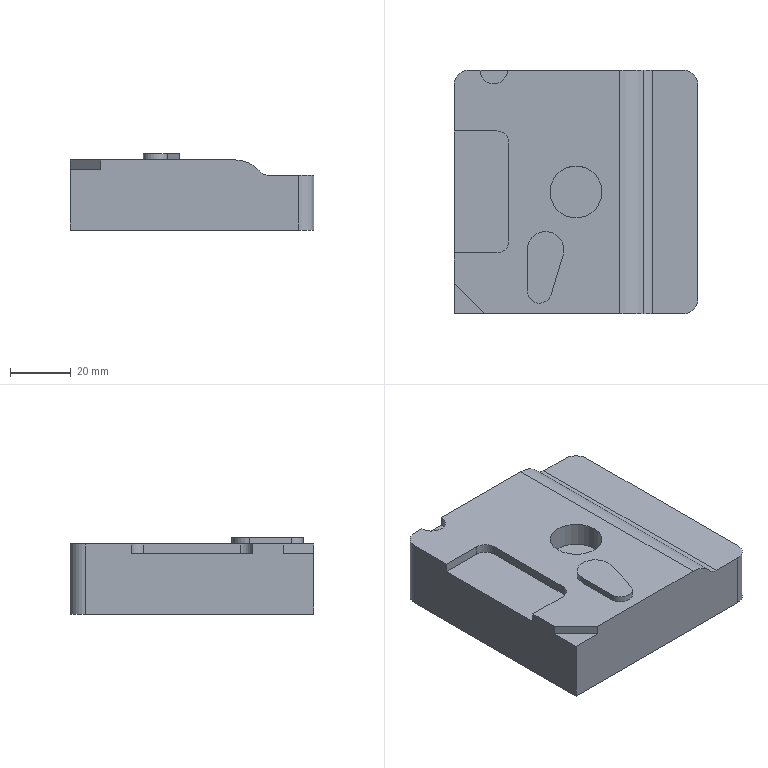Part | NX | 1 solid | 29 faces | box 80 x 80 x 25 mm | volume 135361 mm3 | plane 18 | cylinder 11 | commonest cylinder face diameters 8 x4 10 x3 9 x1 12 x1 17 x1 20 x1
STEP:
#1=CARTESIAN_POINT('',(-35.,40.,0.));
#2=VERTEX_POINT('',#1);
#3=CARTESIAN_POINT('',(-31.5,40.,0.));
#4=VERTEX_POINT('',#3);
#5=CARTESIAN_POINT('',(-40.,40.,0.));
#6=DIRECTION('',(1.,0.,0.));
#7=VECTOR('',#6,1000.);
#8=LINE('',#5,#7);
#9=EDGE_CURVE('',#2,#4,#8,.T.);
#10=ORIENTED_EDGE('',*,*,#9,.F.);
#11=CARTESIAN_POINT('',(-40.,35.,0.));
#12=VERTEX_POINT('',#11);
#13=CARTESIAN_POINT('',(-35.,35.,0.));
#14=DIRECTION('',(0.,0.,1.));
#15=DIRECTION('',(1.,0.,0.));
#16=AXIS2_PLACEMENT_3D('',#13,#14,#15);
#17=CIRCLE('',#16,5.);
#18=EDGE_CURVE('',#2,#12,#17,.T.);
#19=ORIENTED_EDGE('',*,*,#18,.T.);
#20=CARTESIAN_POINT('',(-40.,20.,0.));
#21=VERTEX_POINT('',#20);
#22=CARTESIAN_POINT('',(-40.,-40.,0.));
#23=DIRECTION('',(0.,1.,0.));
#24=VECTOR('',#23,1000.);
#25=LINE('',#22,#24);
#26=EDGE_CURVE('',#21,#12,#25,.T.);
#27=ORIENTED_EDGE('',*,*,#26,.F.);
#28=CARTESIAN_POINT('',(-26.,20.,0.));
#29=VERTEX_POINT('',#28);
#30=CARTESIAN_POINT('',(-22.,20.,0.));
#31=DIRECTION('',(-1.,0.,0.));
#32=VECTOR('',#31,1000.);
#33=LINE('',#30,#32);
#34=EDGE_CURVE('',#29,#21,#33,.T.);
#35=ORIENTED_EDGE('',*,*,#34,.F.);
#36=CARTESIAN_POINT('',(-22.,16.,0.));
#37=VERTEX_POINT('',#36);
#38=CARTESIAN_POINT('',(-26.,16.,0.));
#39=DIRECTION('',(0.,0.,1.));
#40=DIRECTION('',(1.,0.,0.));
#41=AXIS2_PLACEMENT_3D('',#38,#39,#40);
#42=CIRCLE('',#41,4.);
#43=EDGE_CURVE('',#29,#37,#42,.F.);
#44=ORIENTED_EDGE('',*,*,#43,.T.);
#45=CARTESIAN_POINT('',(-22.,-16.,0.));
#46=VERTEX_POINT('',#45);
#47=CARTESIAN_POINT('',(-22.,20.,0.));
#48=DIRECTION('',(0.,-1.,0.));
#49=VECTOR('',#48,1000.);
#50=LINE('',#47,#49);
#51=EDGE_CURVE('',#37,#46,#50,.T.);
#52=ORIENTED_EDGE('',*,*,#51,.T.);
#53=CARTESIAN_POINT('',(-26.,-20.,0.));
#54=VERTEX_POINT('',#53);
#55=CARTESIAN_POINT('',(-26.,-16.,0.));
#56=DIRECTION('',(0.,0.,1.));
#57=DIRECTION('',(1.,0.,0.));
#58=AXIS2_PLACEMENT_3D('',#55,#56,#57);
#59=CIRCLE('',#58,4.);
#60=EDGE_CURVE('',#46,#54,#59,.F.);
#61=ORIENTED_EDGE('',*,*,#60,.T.);
#62=CARTESIAN_POINT('',(-40.,-20.,0.));
#63=VERTEX_POINT('',#62);
#64=CARTESIAN_POINT('',(-22.,-20.,0.));
#65=DIRECTION('',(-1.,0.,0.));
#66=VECTOR('',#65,1000.);
#67=LINE('',#64,#66);
#68=EDGE_CURVE('',#54,#63,#67,.T.);
#69=ORIENTED_EDGE('',*,*,#68,.T.);
#70=CARTESIAN_POINT('',(-40.,-30.,0.));
#71=VERTEX_POINT('',#70);
#72=CARTESIAN_POINT('',(-40.,-40.,0.));
#73=DIRECTION('',(0.,1.,0.));
#74=VECTOR('',#73,1000.);
#75=LINE('',#72,#74);
#76=EDGE_CURVE('',#71,#63,#75,.T.);
#77=ORIENTED_EDGE('',*,*,#76,.F.);
#78=CARTESIAN_POINT('',(-30.,-40.,0.));
#79=VERTEX_POINT('',#78);
#80=CARTESIAN_POINT('',(-30.,-40.,0.));
#81=DIRECTION('',(-0.7071,0.7071,0.));
#82=VECTOR('',#81,1000.);
#83=LINE('',#80,#82);
#84=EDGE_CURVE('',#79,#71,#83,.T.);
#85=ORIENTED_EDGE('',*,*,#84,.F.);
#86=CARTESIAN_POINT('',(14.34,-40.,0.));
#87=VERTEX_POINT('',#86);
#88=CARTESIAN_POINT('',(-40.,-40.,0.));
#89=DIRECTION('',(1.,0.,0.));
#90=VECTOR('',#89,1000.);
#91=LINE('',#88,#90);
#92=EDGE_CURVE('',#79,#87,#91,.T.);
#93=ORIENTED_EDGE('',*,*,#92,.T.);
#94=CARTESIAN_POINT('',(14.34,40.,0.));
#95=VERTEX_POINT('',#94);
#96=CARTESIAN_POINT('',(14.34,-40.,0.));
#97=DIRECTION('',(0.,1.,0.));
#98=VECTOR('',#97,1000.);
#99=LINE('',#96,#98);
#100=EDGE_CURVE('',#87,#95,#99,.T.);
#101=ORIENTED_EDGE('',*,*,#100,.T.);
#102=CARTESIAN_POINT('',(-22.5,40.,0.));
#103=VERTEX_POINT('',#102);
#104=CARTESIAN_POINT('',(-40.,40.,0.));
#105=DIRECTION('',(1.,0.,0.));
#106=VECTOR('',#105,1000.);
#107=LINE('',#104,#106);
#108=EDGE_CURVE('',#103,#95,#107,.T.);
#109=ORIENTED_EDGE('',*,*,#108,.F.);
#110=CARTESIAN_POINT('',(-27.,40.,0.));
#111=DIRECTION('',(0.,0.,-1.));
#112=DIRECTION('',(1.,0.,0.));
#113=AXIS2_PLACEMENT_3D('',#110,#111,#112);
#114=CIRCLE('',#113,4.5);
#115=EDGE_CURVE('',#103,#4,#114,.T.);
#116=ORIENTED_EDGE('',*,*,#115,.T.);
#117=EDGE_LOOP('',(#10,#19,#27,#35,#44,#52,#61,#69,#77,#85,#93,#101,#109,#116));
#118=FACE_BOUND('',#117,.T.);
#119=CARTESIAN_POINT('',(8.5,0.,0.));
#120=VERTEX_POINT('',#119);
#121=CARTESIAN_POINT('',(0.,0.,0.));
#122=DIRECTION('',(0.,0.,1.));
#123=DIRECTION('',(1.,0.,0.));
#124=AXIS2_PLACEMENT_3D('',#121,#122,#123);
#125=CIRCLE('',#124,8.5);
#126=EDGE_CURVE('',#120,#120,#125,.T.);
#127=ORIENTED_EDGE('',*,*,#126,.F.);
#128=EDGE_LOOP('',(#127));
#129=FACE_BOUND('',#128,.T.);
#130=CARTESIAN_POINT('',(-8.172,-33.66,0.));
#131=VERTEX_POINT('',#130);
#132=CARTESIAN_POINT('',(-4.258,-20.74,0.));
#133=VERTEX_POINT('',#132);
#134=CARTESIAN_POINT('',(-8.172,-33.66,0.));
#135=DIRECTION('',(0.2899,0.957,0.));
#136=VECTOR('',#135,1000.);
#137=LINE('',#134,#136);
#138=EDGE_CURVE('',#131,#133,#137,.T.);
#139=ORIENTED_EDGE('',*,*,#138,.F.);
#140=CARTESIAN_POINT('',(-16.,-32.5,0.));
#141=VERTEX_POINT('',#140);
#142=CARTESIAN_POINT('',(-12.,-32.5,0.));
#143=DIRECTION('',(0.,0.,1.));
#144=DIRECTION('',(1.,0.,0.));
#145=AXIS2_PLACEMENT_3D('',#142,#143,#144);
#146=CIRCLE('',#145,4.);
#147=EDGE_CURVE('',#141,#131,#146,.T.);
#148=ORIENTED_EDGE('',*,*,#147,.F.);
#149=CARTESIAN_POINT('',(-16.,-19.,0.));
#150=VERTEX_POINT('',#149);
#151=CARTESIAN_POINT('',(-16.,-19.,0.));
#152=DIRECTION('',(0.,-1.,0.));
#153=VECTOR('',#152,1000.);
#154=LINE('',#151,#153);
#155=EDGE_CURVE('',#150,#141,#154,.T.);
#156=ORIENTED_EDGE('',*,*,#155,.F.);
#157=CARTESIAN_POINT('',(-10.,-19.,0.));
#158=DIRECTION('',(0.,0.,1.));
#159=DIRECTION('',(1.,0.,0.));
#160=AXIS2_PLACEMENT_3D('',#157,#158,#159);
#161=CIRCLE('',#160,6.);
#162=EDGE_CURVE('',#133,#150,#161,.T.);
#163=ORIENTED_EDGE('',*,*,#162,.F.);
#164=EDGE_LOOP('',(#139,#148,#156,#163));
#165=FACE_BOUND('',#164,.T.);
#166=CARTESIAN_POINT('',(-40.,-40.,0.));
#167=DIRECTION('',(0.,0.,1.));
#168=DIRECTION('',(1.,0.,0.));
#169=AXIS2_PLACEMENT_3D('',#166,#167,#168);
#170=PLANE('',#169);
#171=ADVANCED_FACE('',(#118,#129,#165),#170,.T.);
#172=CARTESIAN_POINT('',(35.,40.,-23.));
#173=VERTEX_POINT('',#172);
#174=CARTESIAN_POINT('',(-35.,40.,-23.));
#175=VERTEX_POINT('',#174);
#176=CARTESIAN_POINT('',(40.,40.,-23.));
#177=DIRECTION('',(-1.,0.,0.));
#178=VECTOR('',#177,1000.);
#179=LINE('',#176,#178);
#180=EDGE_CURVE('',#173,#175,#179,.T.);
#181=ORIENTED_EDGE('',*,*,#180,.T.);
#182=CARTESIAN_POINT('',(-35.,40.,0.));
#183=DIRECTION('',(0.,0.,1.));
#184=VECTOR('',#183,1000.);
#185=LINE('',#182,#184);
#186=EDGE_CURVE('',#175,#2,#185,.T.);
#187=ORIENTED_EDGE('',*,*,#186,.T.);
#188=ORIENTED_EDGE('',*,*,#9,.T.);
#189=CARTESIAN_POINT('',(-31.5,40.,-3.));
#190=VERTEX_POINT('',#189);
#191=CARTESIAN_POINT('',(-31.5,40.,-3.));
#192=DIRECTION('',(0.,0.,1.));
#193=VECTOR('',#192,1000.);
#194=LINE('',#191,#193);
#195=EDGE_CURVE('',#190,#4,#194,.T.);
#196=ORIENTED_EDGE('',*,*,#195,.F.);
#197=CARTESIAN_POINT('',(-22.5,40.,-3.));
#198=VERTEX_POINT('',#197);
#199=CARTESIAN_POINT('',(-31.5,40.,-3.));
#200=DIRECTION('',(1.,0.,0.));
#201=VECTOR('',#200,1000.);
#202=LINE('',#199,#201);
#203=EDGE_CURVE('',#190,#198,#202,.T.);
#204=ORIENTED_EDGE('',*,*,#203,.T.);
#205=CARTESIAN_POINT('',(-22.5,40.,-3.));
#206=DIRECTION('',(0.,0.,1.));
#207=VECTOR('',#206,1000.);
#208=LINE('',#205,#207);
#209=EDGE_CURVE('',#198,#103,#208,.T.);
#210=ORIENTED_EDGE('',*,*,#209,.T.);
#211=ORIENTED_EDGE('',*,*,#108,.T.);
#212=CARTESIAN_POINT('',(22.,40.,-3.571));
#213=VERTEX_POINT('',#212);
#214=CARTESIAN_POINT('',(14.34,40.,-10.));
#215=DIRECTION('',(0.,1.,0.));
#216=DIRECTION('',(1.,0.,0.));
#217=AXIS2_PLACEMENT_3D('',#214,#215,#216);
#218=CIRCLE('',#217,10.);
#219=EDGE_CURVE('',#95,#213,#218,.T.);
#220=ORIENTED_EDGE('',*,*,#219,.T.);
#221=CARTESIAN_POINT('',(25.064,40.,-5.));
#222=VERTEX_POINT('',#221);
#223=CARTESIAN_POINT('',(25.064,40.,-1.));
#224=DIRECTION('',(0.,-1.,0.));
#225=DIRECTION('',(1.,0.,0.));
#226=AXIS2_PLACEMENT_3D('',#223,#224,#225);
#227=CIRCLE('',#226,4.);
#228=EDGE_CURVE('',#213,#222,#227,.T.);
#229=ORIENTED_EDGE('',*,*,#228,.T.);
#230=CARTESIAN_POINT('',(35.,40.,-5.));
#231=VERTEX_POINT('',#230);
#232=CARTESIAN_POINT('',(25.064,40.,-5.));
#233=DIRECTION('',(1.,0.,0.));
#234=VECTOR('',#233,1000.);
#235=LINE('',#232,#234);
#236=EDGE_CURVE('',#222,#231,#235,.T.);
#237=ORIENTED_EDGE('',*,*,#236,.T.);
#238=CARTESIAN_POINT('',(35.,40.,-23.));
#239=DIRECTION('',(0.,0.,-1.));
#240=VECTOR('',#239,1000.);
#241=LINE('',#238,#240);
#242=EDGE_CURVE('',#231,#173,#241,.T.);
#243=ORIENTED_EDGE('',*,*,#242,.T.);
#244=EDGE_LOOP('',(#181,#187,#188,#196,#204,#210,#211,#220,#229,#237,#243));
#245=FACE_BOUND('',#244,.T.);
#246=CARTESIAN_POINT('',(25.064,40.,-1.));
#247=DIRECTION('',(0.,-1.,0.));
#248=DIRECTION('',(0.,0.,-1.));
#249=AXIS2_PLACEMENT_3D('',#246,#247,#248);
#250=PLANE('',#249);
#251=ADVANCED_FACE('',(#245),#250,.F.);
#252=ORIENTED_EDGE('',*,*,#26,.T.);
#253=CARTESIAN_POINT('',(-40.,35.,-23.));
#254=VERTEX_POINT('',#253);
#255=CARTESIAN_POINT('',(-40.,35.,-23.));
#256=DIRECTION('',(0.,0.,1.));
#257=VECTOR('',#256,1000.);
#258=LINE('',#255,#257);
#259=EDGE_CURVE('',#12,#254,#258,.F.);
#260=ORIENTED_EDGE('',*,*,#259,.T.);
#261=CARTESIAN_POINT('',(-40.,-40.,-23.));
#262=VERTEX_POINT('',#261);
#263=CARTESIAN_POINT('',(-40.,-40.,-23.));
#264=DIRECTION('',(0.,1.,0.));
#265=VECTOR('',#264,1000.);
#266=LINE('',#263,#265);
#267=EDGE_CURVE('',#262,#254,#266,.T.);
#268=ORIENTED_EDGE('',*,*,#267,.F.);
#269=CARTESIAN_POINT('',(-40.,-40.,-3.));
#270=VERTEX_POINT('',#269);
#271=CARTESIAN_POINT('',(-40.,-40.,-23.));
#272=DIRECTION('',(0.,0.,1.));
#273=VECTOR('',#272,1000.);
#274=LINE('',#271,#273);
#275=EDGE_CURVE('',#262,#270,#274,.T.);
#276=ORIENTED_EDGE('',*,*,#275,.T.);
#277=CARTESIAN_POINT('',(-40.,-30.,-3.));
#278=VERTEX_POINT('',#277);
#279=CARTESIAN_POINT('',(-40.,-30.,-3.));
#280=DIRECTION('',(0.,-1.,0.));
#281=VECTOR('',#280,1000.);
#282=LINE('',#279,#281);
#283=EDGE_CURVE('',#278,#270,#282,.T.);
#284=ORIENTED_EDGE('',*,*,#283,.F.);
#285=CARTESIAN_POINT('',(-40.,-30.,-3.));
#286=DIRECTION('',(0.,0.,1.));
#287=VECTOR('',#286,1000.);
#288=LINE('',#285,#287);
#289=EDGE_CURVE('',#278,#71,#288,.T.);
#290=ORIENTED_EDGE('',*,*,#289,.T.);
#291=ORIENTED_EDGE('',*,*,#76,.T.);
#292=CARTESIAN_POINT('',(-40.,-20.,-3.));
#293=VERTEX_POINT('',#292);
#294=CARTESIAN_POINT('',(-40.,-20.,0.));
#295=DIRECTION('',(0.,0.,-1.));
#296=VECTOR('',#295,1000.);
#297=LINE('',#294,#296);
#298=EDGE_CURVE('',#63,#293,#297,.T.);
#299=ORIENTED_EDGE('',*,*,#298,.T.);
#300=CARTESIAN_POINT('',(-40.,20.,-3.));
#301=VERTEX_POINT('',#300);
#302=CARTESIAN_POINT('',(-40.,-20.,-3.));
#303=DIRECTION('',(0.,1.,0.));
#304=VECTOR('',#303,1000.);
#305=LINE('',#302,#304);
#306=EDGE_CURVE('',#293,#301,#305,.T.);
#307=ORIENTED_EDGE('',*,*,#306,.T.);
#308=CARTESIAN_POINT('',(-40.,20.,-3.));
#309=DIRECTION('',(0.,0.,1.));
#310=VECTOR('',#309,1000.);
#311=LINE('',#308,#310);
#312=EDGE_CURVE('',#301,#21,#311,.T.);
#313=ORIENTED_EDGE('',*,*,#312,.T.);
#314=EDGE_LOOP('',(#252,#260,#268,#276,#284,#290,#291,#299,#307,#313));
#315=FACE_BOUND('',#314,.T.);
#316=CARTESIAN_POINT('',(-40.,-40.,-23.));
#317=DIRECTION('',(-1.,0.,0.));
#318=DIRECTION('',(0.,0.,1.));
#319=AXIS2_PLACEMENT_3D('',#316,#317,#318);
#320=PLANE('',#319);
#321=ADVANCED_FACE('',(#315),#320,.T.);
#322=ORIENTED_EDGE('',*,*,#228,.F.);
#323=CARTESIAN_POINT('',(22.,-40.,-3.571));
#324=VERTEX_POINT('',#323);
#325=CARTESIAN_POINT('',(22.,-40.,-3.571));
#326=DIRECTION('',(0.,1.,0.));
#327=VECTOR('',#326,1000.);
#328=LINE('',#325,#327);
#329=EDGE_CURVE('',#324,#213,#328,.T.);
#330=ORIENTED_EDGE('',*,*,#329,.F.);
#331=CARTESIAN_POINT('',(25.064,-40.,-5.));
#332=VERTEX_POINT('',#331);
#333=CARTESIAN_POINT('',(25.064,-40.,-1.));
#334=DIRECTION('',(0.,-1.,0.));
#335=DIRECTION('',(1.,0.,0.));
#336=AXIS2_PLACEMENT_3D('',#333,#334,#335);
#337=CIRCLE('',#336,4.);
#338=EDGE_CURVE('',#324,#332,#337,.T.);
#339=ORIENTED_EDGE('',*,*,#338,.T.);
#340=CARTESIAN_POINT('',(25.064,-40.,-5.));
#341=DIRECTION('',(0.,1.,0.));
#342=VECTOR('',#341,1000.);
#343=LINE('',#340,#342);
#344=EDGE_CURVE('',#332,#222,#343,.T.);
#345=ORIENTED_EDGE('',*,*,#344,.T.);
#346=EDGE_LOOP('',(#322,#330,#339,#345));
#347=FACE_BOUND('',#346,.T.);
#348=CARTESIAN_POINT('',(25.064,-40.,-1.));
#349=DIRECTION('',(0.,1.,0.));
#350=DIRECTION('',(0.,0.,1.));
#351=AXIS2_PLACEMENT_3D('',#348,#349,#350);
#352=CYLINDRICAL_SURFACE('',#351,4.);
#353=ADVANCED_FACE('',(#347),#352,.F.);
#354=CARTESIAN_POINT('',(40.,-35.,-5.));
#355=VERTEX_POINT('',#354);
#356=CARTESIAN_POINT('',(40.,35.,-5.));
#357=VERTEX_POINT('',#356);
#358=CARTESIAN_POINT('',(40.,-40.,-5.));
#359=DIRECTION('',(0.,1.,0.));
#360=VECTOR('',#359,1000.);
#361=LINE('',#358,#360);
#362=EDGE_CURVE('',#355,#357,#361,.T.);
#363=ORIENTED_EDGE('',*,*,#362,.T.);
#364=CARTESIAN_POINT('',(35.,35.,-5.));
#365=DIRECTION('',(0.,0.,1.));
#366=DIRECTION('',(1.,0.,0.));
#367=AXIS2_PLACEMENT_3D('',#364,#365,#366);
#368=CIRCLE('',#367,5.);
#369=EDGE_CURVE('',#357,#231,#368,.T.);
#370=ORIENTED_EDGE('',*,*,#369,.T.);
#371=ORIENTED_EDGE('',*,*,#236,.F.);
#372=ORIENTED_EDGE('',*,*,#344,.F.);
#373=CARTESIAN_POINT('',(35.,-40.,-5.));
#374=VERTEX_POINT('',#373);
#375=CARTESIAN_POINT('',(25.064,-40.,-5.));
#376=DIRECTION('',(1.,0.,0.));
#377=VECTOR('',#376,1000.);
#378=LINE('',#375,#377);
#379=EDGE_CURVE('',#332,#374,#378,.T.);
#380=ORIENTED_EDGE('',*,*,#379,.T.);
#381=CARTESIAN_POINT('',(35.,-35.,-5.));
#382=DIRECTION('',(0.,0.,1.));
#383=DIRECTION('',(1.,0.,0.));
#384=AXIS2_PLACEMENT_3D('',#381,#382,#383);
#385=CIRCLE('',#384,5.);
#386=EDGE_CURVE('',#374,#355,#385,.T.);
#387=ORIENTED_EDGE('',*,*,#386,.T.);
#388=EDGE_LOOP('',(#363,#370,#371,#372,#380,#387));
#389=FACE_BOUND('',#388,.T.);
#390=CARTESIAN_POINT('',(25.064,-40.,-5.));
#391=DIRECTION('',(0.,0.,1.));
#392=DIRECTION('',(1.,0.,0.));
#393=AXIS2_PLACEMENT_3D('',#390,#391,#392);
#394=PLANE('',#393);
#395=ADVANCED_FACE('',(#389),#394,.T.);
#396=CARTESIAN_POINT('',(40.,-35.,-23.));
#397=VERTEX_POINT('',#396);
#398=CARTESIAN_POINT('',(40.,35.,-23.));
#399=VERTEX_POINT('',#398);
#400=CARTESIAN_POINT('',(40.,-40.,-23.));
#401=DIRECTION('',(0.,1.,0.));
#402=VECTOR('',#401,1000.);
#403=LINE('',#400,#402);
#404=EDGE_CURVE('',#397,#399,#403,.T.);
#405=ORIENTED_EDGE('',*,*,#404,.T.);
#406=CARTESIAN_POINT('',(40.,35.,-5.));
#407=DIRECTION('',(0.,0.,-1.));
#408=VECTOR('',#407,1000.);
#409=LINE('',#406,#408);
#410=EDGE_CURVE('',#399,#357,#409,.F.);
#411=ORIENTED_EDGE('',*,*,#410,.T.);
#412=ORIENTED_EDGE('',*,*,#362,.F.);
#413=CARTESIAN_POINT('',(40.,-35.,-5.));
#414=DIRECTION('',(0.,0.,-1.));
#415=VECTOR('',#414,1000.);
#416=LINE('',#413,#415);
#417=EDGE_CURVE('',#355,#397,#416,.T.);
#418=ORIENTED_EDGE('',*,*,#417,.T.);
#419=EDGE_LOOP('',(#405,#411,#412,#418));
#420=FACE_BOUND('',#419,.T.);
#421=CARTESIAN_POINT('',(40.,-40.,-5.));
#422=DIRECTION('',(1.,0.,0.));
#423=DIRECTION('',(0.,0.,-1.));
#424=AXIS2_PLACEMENT_3D('',#421,#422,#423);
#425=PLANE('',#424);
#426=ADVANCED_FACE('',(#420),#425,.T.);
#427=ORIENTED_EDGE('',*,*,#267,.T.);
#428=CARTESIAN_POINT('',(-35.,35.,-23.));
#429=DIRECTION('',(0.,0.,-1.));
#430=DIRECTION('',(-1.,0.,0.));
#431=AXIS2_PLACEMENT_3D('',#428,#429,#430);
#432=CIRCLE('',#431,5.);
#433=EDGE_CURVE('',#254,#175,#432,.T.);
#434=ORIENTED_EDGE('',*,*,#433,.T.);
#435=ORIENTED_EDGE('',*,*,#180,.F.);
#436=CARTESIAN_POINT('',(35.,35.,-23.));
#437=DIRECTION('',(0.,0.,-1.));
#438=DIRECTION('',(-1.,0.,0.));
#439=AXIS2_PLACEMENT_3D('',#436,#437,#438);
#440=CIRCLE('',#439,5.);
#441=EDGE_CURVE('',#173,#399,#440,.T.);
#442=ORIENTED_EDGE('',*,*,#441,.T.);
#443=ORIENTED_EDGE('',*,*,#404,.F.);
#444=CARTESIAN_POINT('',(35.,-40.,-23.));
#445=VERTEX_POINT('',#444);
#446=CARTESIAN_POINT('',(35.,-35.,-23.));
#447=DIRECTION('',(0.,0.,-1.));
#448=DIRECTION('',(-1.,0.,0.));
#449=AXIS2_PLACEMENT_3D('',#446,#447,#448);
#450=CIRCLE('',#449,5.);
#451=EDGE_CURVE('',#397,#445,#450,.T.);
#452=ORIENTED_EDGE('',*,*,#451,.T.);
#453=CARTESIAN_POINT('',(40.,-40.,-23.));
#454=DIRECTION('',(-1.,0.,0.));
#455=VECTOR('',#454,1000.);
#456=LINE('',#453,#455);
#457=EDGE_CURVE('',#445,#262,#456,.T.);
#458=ORIENTED_EDGE('',*,*,#457,.T.);
#459=EDGE_LOOP('',(#427,#434,#435,#442,#443,#452,#458));
#460=FACE_BOUND('',#459,.T.);
#461=CARTESIAN_POINT('',(40.,-40.,-23.));
#462=DIRECTION('',(0.,0.,-1.));
#463=DIRECTION('',(-1.,0.,0.));
#464=AXIS2_PLACEMENT_3D('',#461,#462,#463);
#465=PLANE('',#464);
#466=ADVANCED_FACE('',(#460),#465,.T.);
#467=ORIENTED_EDGE('',*,*,#219,.F.);
#468=ORIENTED_EDGE('',*,*,#100,.F.);
#469=CARTESIAN_POINT('',(14.34,-40.,-10.));
#470=DIRECTION('',(0.,1.,0.));
#471=DIRECTION('',(1.,0.,0.));
#472=AXIS2_PLACEMENT_3D('',#469,#470,#471);
#473=CIRCLE('',#472,10.);
#474=EDGE_CURVE('',#87,#324,#473,.T.);
#475=ORIENTED_EDGE('',*,*,#474,.T.);
#476=ORIENTED_EDGE('',*,*,#329,.T.);
#477=EDGE_LOOP('',(#467,#468,#475,#476));
#478=FACE_BOUND('',#477,.T.);
#479=CARTESIAN_POINT('',(14.34,-40.,-10.));
#480=DIRECTION('',(0.,1.,0.));
#481=DIRECTION('',(0.,0.,1.));
#482=AXIS2_PLACEMENT_3D('',#479,#480,#481);
#483=CYLINDRICAL_SURFACE('',#482,10.);
#484=ADVANCED_FACE('',(#478),#483,.T.);
#485=ORIENTED_EDGE('',*,*,#457,.F.);
#486=CARTESIAN_POINT('',(35.,-40.,-1.));
#487=DIRECTION('',(0.,0.,-1.));
#488=VECTOR('',#487,1000.);
#489=LINE('',#486,#488);
#490=EDGE_CURVE('',#445,#374,#489,.F.);
#491=ORIENTED_EDGE('',*,*,#490,.T.);
#492=ORIENTED_EDGE('',*,*,#379,.F.);
#493=ORIENTED_EDGE('',*,*,#338,.F.);
#494=ORIENTED_EDGE('',*,*,#474,.F.);
#495=ORIENTED_EDGE('',*,*,#92,.F.);
#496=CARTESIAN_POINT('',(-30.,-40.,-3.));
#497=VERTEX_POINT('',#496);
#498=CARTESIAN_POINT('',(-30.,-40.,-3.));
#499=DIRECTION('',(0.,0.,1.));
#500=VECTOR('',#499,1000.);
#501=LINE('',#498,#500);
#502=EDGE_CURVE('',#497,#79,#501,.T.);
#503=ORIENTED_EDGE('',*,*,#502,.F.);
#504=CARTESIAN_POINT('',(-40.,-40.,-3.));
#505=DIRECTION('',(1.,0.,0.));
#506=VECTOR('',#505,1000.);
#507=LINE('',#504,#506);
#508=EDGE_CURVE('',#270,#497,#507,.T.);
#509=ORIENTED_EDGE('',*,*,#508,.F.);
#510=ORIENTED_EDGE('',*,*,#275,.F.);
#511=EDGE_LOOP('',(#485,#491,#492,#493,#494,#495,#503,#509,#510));
#512=FACE_BOUND('',#511,.T.);
#513=CARTESIAN_POINT('',(25.064,-40.,-1.));
#514=DIRECTION('',(0.,-1.,0.));
#515=DIRECTION('',(0.,0.,-1.));
#516=AXIS2_PLACEMENT_3D('',#513,#514,#515);
#517=PLANE('',#516);
#518=ADVANCED_FACE('',(#512),#517,.T.);
#519=CARTESIAN_POINT('',(8.5,0.,-8.));
#520=VERTEX_POINT('',#519);
#521=CARTESIAN_POINT('',(0.,0.,-8.));
#522=DIRECTION('',(0.,0.,1.));
#523=DIRECTION('',(1.,0.,0.));
#524=AXIS2_PLACEMENT_3D('',#521,#522,#523);
#525=CIRCLE('',#524,8.5);
#526=EDGE_CURVE('',#520,#520,#525,.T.);
#527=ORIENTED_EDGE('',*,*,#526,.F.);
#528=EDGE_LOOP('',(#527));
#529=FACE_BOUND('',#528,.T.);
#530=ORIENTED_EDGE('',*,*,#126,.T.);
#531=EDGE_LOOP('',(#530));
#532=FACE_BOUND('',#531,.T.);
#533=CARTESIAN_POINT('',(0.,0.,-8.));
#534=DIRECTION('',(0.,0.,1.));
#535=DIRECTION('',(1.,0.,0.));
#536=AXIS2_PLACEMENT_3D('',#533,#534,#535);
#537=CYLINDRICAL_SURFACE('',#536,8.5);
#538=ADVANCED_FACE('',(#529,#532),#537,.F.);
#539=ORIENTED_EDGE('',*,*,#526,.T.);
#540=EDGE_LOOP('',(#539));
#541=FACE_BOUND('',#540,.T.);
#542=CARTESIAN_POINT('',(0.,0.,-8.));
#543=DIRECTION('',(0.,0.,1.));
#544=DIRECTION('',(1.,0.,0.));
#545=AXIS2_PLACEMENT_3D('',#542,#543,#544);
#546=PLANE('',#545);
#547=ADVANCED_FACE('',(#541),#546,.T.);
#548=CARTESIAN_POINT('',(-26.,-20.,-3.));
#549=VERTEX_POINT('',#548);
#550=CARTESIAN_POINT('',(-22.,-20.,-3.));
#551=DIRECTION('',(-1.,0.,0.));
#552=VECTOR('',#551,1000.);
#553=LINE('',#550,#552);
#554=EDGE_CURVE('',#549,#293,#553,.T.);
#555=ORIENTED_EDGE('',*,*,#554,.F.);
#556=CARTESIAN_POINT('',(-22.,-16.,-3.));
#557=VERTEX_POINT('',#556);
#558=CARTESIAN_POINT('',(-26.,-16.,-3.));
#559=DIRECTION('',(0.,0.,1.));
#560=DIRECTION('',(0.,-1.,0.));
#561=AXIS2_PLACEMENT_3D('',#558,#559,#560);
#562=CIRCLE('',#561,4.);
#563=EDGE_CURVE('',#549,#557,#562,.T.);
#564=ORIENTED_EDGE('',*,*,#563,.T.);
#565=CARTESIAN_POINT('',(-22.,16.,-3.));
#566=VERTEX_POINT('',#565);
#567=CARTESIAN_POINT('',(-22.,-20.,-3.));
#568=DIRECTION('',(0.,1.,0.));
#569=VECTOR('',#568,1000.);
#570=LINE('',#567,#569);
#571=EDGE_CURVE('',#557,#566,#570,.T.);
#572=ORIENTED_EDGE('',*,*,#571,.T.);
#573=CARTESIAN_POINT('',(-26.,20.,-3.));
#574=VERTEX_POINT('',#573);
#575=CARTESIAN_POINT('',(-26.,16.,-3.));
#576=DIRECTION('',(0.,0.,1.));
#577=DIRECTION('',(0.,-1.,0.));
#578=AXIS2_PLACEMENT_3D('',#575,#576,#577);
#579=CIRCLE('',#578,4.);
#580=EDGE_CURVE('',#566,#574,#579,.T.);
#581=ORIENTED_EDGE('',*,*,#580,.T.);
#582=CARTESIAN_POINT('',(-22.,20.,-3.));
#583=DIRECTION('',(-1.,0.,0.));
#584=VECTOR('',#583,1000.);
#585=LINE('',#582,#584);
#586=EDGE_CURVE('',#574,#301,#585,.T.);
#587=ORIENTED_EDGE('',*,*,#586,.T.);
#588=ORIENTED_EDGE('',*,*,#306,.F.);
#589=EDGE_LOOP('',(#555,#564,#572,#581,#587,#588));
#590=FACE_BOUND('',#589,.T.);
#591=CARTESIAN_POINT('',(-22.,-20.,-3.));
#592=DIRECTION('',(0.,0.,1.));
#593=DIRECTION('',(0.,-1.,0.));
#594=AXIS2_PLACEMENT_3D('',#591,#592,#593);
#595=PLANE('',#594);
#596=ADVANCED_FACE('',(#590),#595,.T.);
#597=ORIENTED_EDGE('',*,*,#586,.F.);
#598=CARTESIAN_POINT('',(-26.,20.,-3.));
#599=DIRECTION('',(0.,0.,1.));
#600=VECTOR('',#599,1000.);
#601=LINE('',#598,#600);
#602=EDGE_CURVE('',#574,#29,#601,.T.);
#603=ORIENTED_EDGE('',*,*,#602,.T.);
#604=ORIENTED_EDGE('',*,*,#34,.T.);
#605=ORIENTED_EDGE('',*,*,#312,.F.);
#606=EDGE_LOOP('',(#597,#603,#604,#605));
#607=FACE_BOUND('',#606,.T.);
#608=CARTESIAN_POINT('',(-22.,20.,-3.));
#609=DIRECTION('',(0.,-1.,0.));
#610=DIRECTION('',(0.,0.,-1.));
#611=AXIS2_PLACEMENT_3D('',#608,#609,#610);
#612=PLANE('',#611);
#613=ADVANCED_FACE('',(#607),#612,.T.);
#614=ORIENTED_EDGE('',*,*,#68,.F.);
#615=CARTESIAN_POINT('',(-26.,-20.,0.));
#616=DIRECTION('',(0.,0.,-1.));
#617=VECTOR('',#616,1000.);
#618=LINE('',#615,#617);
#619=EDGE_CURVE('',#54,#549,#618,.T.);
#620=ORIENTED_EDGE('',*,*,#619,.T.);
#621=ORIENTED_EDGE('',*,*,#554,.T.);
#622=ORIENTED_EDGE('',*,*,#298,.F.);
#623=EDGE_LOOP('',(#614,#620,#621,#622));
#624=FACE_BOUND('',#623,.T.);
#625=CARTESIAN_POINT('',(-22.,-20.,0.));
#626=DIRECTION('',(0.,1.,0.));
#627=DIRECTION('',(0.,0.,1.));
#628=AXIS2_PLACEMENT_3D('',#625,#626,#627);
#629=PLANE('',#628);
#630=ADVANCED_FACE('',(#624),#629,.T.);
#631=ORIENTED_EDGE('',*,*,#571,.F.);
#632=CARTESIAN_POINT('',(-22.,-16.,-3.));
#633=DIRECTION('',(0.,0.,-1.));
#634=VECTOR('',#633,1000.);
#635=LINE('',#632,#634);
#636=EDGE_CURVE('',#557,#46,#635,.F.);
#637=ORIENTED_EDGE('',*,*,#636,.T.);
#638=ORIENTED_EDGE('',*,*,#51,.F.);
#639=CARTESIAN_POINT('',(-22.,16.,-3.));
#640=DIRECTION('',(0.,0.,1.));
#641=VECTOR('',#640,1000.);
#642=LINE('',#639,#641);
#643=EDGE_CURVE('',#37,#566,#642,.F.);
#644=ORIENTED_EDGE('',*,*,#643,.T.);
#645=EDGE_LOOP('',(#631,#637,#638,#644));
#646=FACE_BOUND('',#645,.T.);
#647=CARTESIAN_POINT('',(-22.,20.,-3.));
#648=DIRECTION('',(1.,0.,0.));
#649=DIRECTION('',(0.,0.,-1.));
#650=AXIS2_PLACEMENT_3D('',#647,#648,#649);
#651=PLANE('',#650);
#652=ADVANCED_FACE('',(#646),#651,.F.);
#653=ORIENTED_EDGE('',*,*,#60,.F.);
#654=ORIENTED_EDGE('',*,*,#636,.F.);
#655=ORIENTED_EDGE('',*,*,#563,.F.);
#656=ORIENTED_EDGE('',*,*,#619,.F.);
#657=EDGE_LOOP('',(#653,#654,#655,#656));
#658=FACE_BOUND('',#657,.T.);
#659=CARTESIAN_POINT('',(-26.,-16.,0.));
#660=DIRECTION('',(0.,0.,-1.));
#661=DIRECTION('',(-1.,0.,0.));
#662=AXIS2_PLACEMENT_3D('',#659,#660,#661);
#663=CYLINDRICAL_SURFACE('',#662,4.);
#664=ADVANCED_FACE('',(#658),#663,.F.);
#665=ORIENTED_EDGE('',*,*,#580,.F.);
#666=ORIENTED_EDGE('',*,*,#643,.F.);
#667=ORIENTED_EDGE('',*,*,#43,.F.);
#668=ORIENTED_EDGE('',*,*,#602,.F.);
#669=EDGE_LOOP('',(#665,#666,#667,#668));
#670=FACE_BOUND('',#669,.T.);
#671=CARTESIAN_POINT('',(-26.,16.,-3.));
#672=DIRECTION('',(0.,0.,1.));
#673=DIRECTION('',(1.,0.,0.));
#674=AXIS2_PLACEMENT_3D('',#671,#672,#673);
#675=CYLINDRICAL_SURFACE('',#674,4.);
#676=ADVANCED_FACE('',(#670),#675,.F.);
#677=ORIENTED_EDGE('',*,*,#84,.T.);
#678=ORIENTED_EDGE('',*,*,#289,.F.);
#679=CARTESIAN_POINT('',(-30.,-40.,-3.));
#680=DIRECTION('',(-0.7071,0.7071,0.));
#681=VECTOR('',#680,1000.);
#682=LINE('',#679,#681);
#683=EDGE_CURVE('',#497,#278,#682,.T.);
#684=ORIENTED_EDGE('',*,*,#683,.F.);
#685=ORIENTED_EDGE('',*,*,#502,.T.);
#686=EDGE_LOOP('',(#677,#678,#684,#685));
#687=FACE_BOUND('',#686,.T.);
#688=CARTESIAN_POINT('',(-30.,-40.,-3.));
#689=DIRECTION('',(0.7071,0.7071,0.));
#690=DIRECTION('',(-0.7071,0.7071,0.));
#691=AXIS2_PLACEMENT_3D('',#688,#689,#690);
#692=PLANE('',#691);
#693=ADVANCED_FACE('',(#687),#692,.F.);
#694=ORIENTED_EDGE('',*,*,#508,.T.);
#695=ORIENTED_EDGE('',*,*,#683,.T.);
#696=ORIENTED_EDGE('',*,*,#283,.T.);
#697=EDGE_LOOP('',(#694,#695,#696));
#698=FACE_BOUND('',#697,.T.);
#699=CARTESIAN_POINT('',(-40.,-40.,-3.));
#700=DIRECTION('',(0.,0.,-1.));
#701=DIRECTION('',(-1.,0.,0.));
#702=AXIS2_PLACEMENT_3D('',#699,#700,#701);
#703=PLANE('',#702);
#704=ADVANCED_FACE('',(#698),#703,.F.);
#705=ORIENTED_EDGE('',*,*,#115,.F.);
#706=ORIENTED_EDGE('',*,*,#209,.F.);
#707=CARTESIAN_POINT('',(-27.,40.,-3.));
#708=DIRECTION('',(0.,0.,-1.));
#709=DIRECTION('',(1.,0.,0.));
#710=AXIS2_PLACEMENT_3D('',#707,#708,#709);
#711=CIRCLE('',#710,4.5);
#712=EDGE_CURVE('',#198,#190,#711,.T.);
#713=ORIENTED_EDGE('',*,*,#712,.T.);
#714=ORIENTED_EDGE('',*,*,#195,.T.);
#715=EDGE_LOOP('',(#705,#706,#713,#714));
#716=FACE_BOUND('',#715,.T.);
#717=CARTESIAN_POINT('',(-27.,40.,-3.));
#718=DIRECTION('',(0.,0.,1.));
#719=DIRECTION('',(1.,0.,0.));
#720=AXIS2_PLACEMENT_3D('',#717,#718,#719);
#721=CYLINDRICAL_SURFACE('',#720,4.5);
#722=ADVANCED_FACE('',(#716),#721,.F.);
#723=ORIENTED_EDGE('',*,*,#712,.F.);
#724=ORIENTED_EDGE('',*,*,#203,.F.);
#725=EDGE_LOOP('',(#723,#724));
#726=FACE_BOUND('',#725,.T.);
#727=CARTESIAN_POINT('',(-27.,40.,-3.));
#728=DIRECTION('',(0.,0.,-1.));
#729=DIRECTION('',(-1.,0.,0.));
#730=AXIS2_PLACEMENT_3D('',#727,#728,#729);
#731=PLANE('',#730);
#732=ADVANCED_FACE('',(#726),#731,.F.);
#733=ORIENTED_EDGE('',*,*,#147,.T.);
#734=CARTESIAN_POINT('',(-8.172,-33.66,2.));
#735=VERTEX_POINT('',#734);
#736=CARTESIAN_POINT('',(-8.172,-33.66,2.));
#737=DIRECTION('',(0.,0.,-1.));
#738=VECTOR('',#737,1000.);
#739=LINE('',#736,#738);
#740=EDGE_CURVE('',#735,#131,#739,.T.);
#741=ORIENTED_EDGE('',*,*,#740,.F.);
#742=CARTESIAN_POINT('',(-16.,-32.5,2.));
#743=VERTEX_POINT('',#742);
#744=CARTESIAN_POINT('',(-12.,-32.5,2.));
#745=DIRECTION('',(0.,0.,1.));
#746=DIRECTION('',(1.,0.,0.));
#747=AXIS2_PLACEMENT_3D('',#744,#745,#746);
#748=CIRCLE('',#747,4.);
#749=EDGE_CURVE('',#743,#735,#748,.T.);
#750=ORIENTED_EDGE('',*,*,#749,.F.);
#751=CARTESIAN_POINT('',(-16.,-32.5,2.));
#752=DIRECTION('',(0.,0.,-1.));
#753=VECTOR('',#752,1000.);
#754=LINE('',#751,#753);
#755=EDGE_CURVE('',#743,#141,#754,.T.);
#756=ORIENTED_EDGE('',*,*,#755,.T.);
#757=EDGE_LOOP('',(#733,#741,#750,#756));
#758=FACE_BOUND('',#757,.T.);
#759=CARTESIAN_POINT('',(-12.,-32.5,2.));
#760=DIRECTION('',(0.,0.,-1.));
#761=DIRECTION('',(-1.,0.,0.));
#762=AXIS2_PLACEMENT_3D('',#759,#760,#761);
#763=CYLINDRICAL_SURFACE('',#762,4.);
#764=ADVANCED_FACE('',(#758),#763,.T.);
#765=ORIENTED_EDGE('',*,*,#138,.T.);
#766=CARTESIAN_POINT('',(-4.258,-20.74,2.));
#767=VERTEX_POINT('',#766);
#768=CARTESIAN_POINT('',(-4.258,-20.74,2.));
#769=DIRECTION('',(0.,0.,-1.));
#770=VECTOR('',#769,1000.);
#771=LINE('',#768,#770);
#772=EDGE_CURVE('',#767,#133,#771,.T.);
#773=ORIENTED_EDGE('',*,*,#772,.F.);
#774=CARTESIAN_POINT('',(-8.172,-33.66,2.));
#775=DIRECTION('',(0.2899,0.957,0.));
#776=VECTOR('',#775,1000.);
#777=LINE('',#774,#776);
#778=EDGE_CURVE('',#735,#767,#777,.T.);
#779=ORIENTED_EDGE('',*,*,#778,.F.);
#780=ORIENTED_EDGE('',*,*,#740,.T.);
#781=EDGE_LOOP('',(#765,#773,#779,#780));
#782=FACE_BOUND('',#781,.T.);
#783=CARTESIAN_POINT('',(-8.172,-33.66,2.));
#784=DIRECTION('',(-0.957,0.2899,0.));
#785=DIRECTION('',(-0.2899,-0.957,0.));
#786=AXIS2_PLACEMENT_3D('',#783,#784,#785);
#787=PLANE('',#786);
#788=ADVANCED_FACE('',(#782),#787,.F.);
#789=ORIENTED_EDGE('',*,*,#162,.T.);
#790=CARTESIAN_POINT('',(-16.,-19.,2.));
#791=VERTEX_POINT('',#790);
#792=CARTESIAN_POINT('',(-16.,-19.,2.));
#793=DIRECTION('',(0.,0.,-1.));
#794=VECTOR('',#793,1000.);
#795=LINE('',#792,#794);
#796=EDGE_CURVE('',#791,#150,#795,.T.);
#797=ORIENTED_EDGE('',*,*,#796,.F.);
#798=CARTESIAN_POINT('',(-10.,-19.,2.));
#799=DIRECTION('',(0.,0.,1.));
#800=DIRECTION('',(1.,0.,0.));
#801=AXIS2_PLACEMENT_3D('',#798,#799,#800);
#802=CIRCLE('',#801,6.);
#803=EDGE_CURVE('',#767,#791,#802,.T.);
#804=ORIENTED_EDGE('',*,*,#803,.F.);
#805=ORIENTED_EDGE('',*,*,#772,.T.);
#806=EDGE_LOOP('',(#789,#797,#804,#805));
#807=FACE_BOUND('',#806,.T.);
#808=CARTESIAN_POINT('',(-10.,-19.,2.));
#809=DIRECTION('',(0.,0.,-1.));
#810=DIRECTION('',(-1.,0.,0.));
#811=AXIS2_PLACEMENT_3D('',#808,#809,#810);
#812=CYLINDRICAL_SURFACE('',#811,6.);
#813=ADVANCED_FACE('',(#807),#812,.T.);
#814=ORIENTED_EDGE('',*,*,#155,.T.);
#815=ORIENTED_EDGE('',*,*,#755,.F.);
#816=CARTESIAN_POINT('',(-16.,-19.,2.));
#817=DIRECTION('',(0.,-1.,0.));
#818=VECTOR('',#817,1000.);
#819=LINE('',#816,#818);
#820=EDGE_CURVE('',#791,#743,#819,.T.);
#821=ORIENTED_EDGE('',*,*,#820,.F.);
#822=ORIENTED_EDGE('',*,*,#796,.T.);
#823=EDGE_LOOP('',(#814,#815,#821,#822));
#824=FACE_BOUND('',#823,.T.);
#825=CARTESIAN_POINT('',(-16.,-19.,2.));
#826=DIRECTION('',(1.,0.,0.));
#827=DIRECTION('',(0.,0.,-1.));
#828=AXIS2_PLACEMENT_3D('',#825,#826,#827);
#829=PLANE('',#828);
#830=ADVANCED_FACE('',(#824),#829,.F.);
#831=ORIENTED_EDGE('',*,*,#749,.T.);
#832=ORIENTED_EDGE('',*,*,#778,.T.);
#833=ORIENTED_EDGE('',*,*,#803,.T.);
#834=ORIENTED_EDGE('',*,*,#820,.T.);
#835=EDGE_LOOP('',(#831,#832,#833,#834));
#836=FACE_BOUND('',#835,.T.);
#837=CARTESIAN_POINT('',(-12.,-32.5,2.));
#838=DIRECTION('',(0.,0.,1.));
#839=DIRECTION('',(1.,0.,0.));
#840=AXIS2_PLACEMENT_3D('',#837,#838,#839);
#841=PLANE('',#840);
#842=ADVANCED_FACE('',(#836),#841,.T.);
#843=ORIENTED_EDGE('',*,*,#433,.F.);
#844=ORIENTED_EDGE('',*,*,#259,.F.);
#845=ORIENTED_EDGE('',*,*,#18,.F.);
#846=ORIENTED_EDGE('',*,*,#186,.F.);
#847=EDGE_LOOP('',(#843,#844,#845,#846));
#848=FACE_BOUND('',#847,.T.);
#849=CARTESIAN_POINT('',(-35.,35.,-1.));
#850=DIRECTION('',(0.,0.,-1.));
#851=DIRECTION('',(-1.,0.,0.));
#852=AXIS2_PLACEMENT_3D('',#849,#850,#851);
#853=CYLINDRICAL_SURFACE('',#852,5.);
#854=ADVANCED_FACE('',(#848),#853,.T.);
#855=ORIENTED_EDGE('',*,*,#369,.F.);
#856=ORIENTED_EDGE('',*,*,#410,.F.);
#857=ORIENTED_EDGE('',*,*,#441,.F.);
#858=ORIENTED_EDGE('',*,*,#242,.F.);
#859=EDGE_LOOP('',(#855,#856,#857,#858));
#860=FACE_BOUND('',#859,.T.);
#861=CARTESIAN_POINT('',(35.,35.,-1.));
#862=DIRECTION('',(0.,0.,1.));
#863=DIRECTION('',(1.,0.,0.));
#864=AXIS2_PLACEMENT_3D('',#861,#862,#863);
#865=CYLINDRICAL_SURFACE('',#864,5.);
#866=ADVANCED_FACE('',(#860),#865,.T.);
#867=ORIENTED_EDGE('',*,*,#386,.F.);
#868=ORIENTED_EDGE('',*,*,#490,.F.);
#869=ORIENTED_EDGE('',*,*,#451,.F.);
#870=ORIENTED_EDGE('',*,*,#417,.F.);
#871=EDGE_LOOP('',(#867,#868,#869,#870));
#872=FACE_BOUND('',#871,.T.);
#873=CARTESIAN_POINT('',(35.,-35.,-5.));
#874=DIRECTION('',(0.,0.,-1.));
#875=DIRECTION('',(-1.,0.,0.));
#876=AXIS2_PLACEMENT_3D('',#873,#874,#875);
#877=CYLINDRICAL_SURFACE('',#876,5.);
#878=ADVANCED_FACE('',(#872),#877,.T.);
#879=CLOSED_SHELL('',(#171,#251,#321,#353,#395,#426,#466,#484,#518,#538,#547,#596,#613,#630,#652,#664,#676,#693,#704,#722,#732,#764,#788,#813,#830,#842,#854,#866,#878));
#880=MANIFOLD_SOLID_BREP('',#879);
#881=(LENGTH_UNIT()NAMED_UNIT(*)SI_UNIT(.MILLI.,.METRE.));
#882=UNCERTAINTY_MEASURE_WITH_UNIT(LENGTH_MEASURE(0.00001),#881,'','');
#883=(NAMED_UNIT(*)PLANE_ANGLE_UNIT()SI_UNIT($,.RADIAN.));
#884=(NAMED_UNIT(*)SI_UNIT($,.STERADIAN.)SOLID_ANGLE_UNIT());
#885=(GEOMETRIC_REPRESENTATION_CONTEXT(3)GLOBAL_UNCERTAINTY_ASSIGNED_CONTEXT((#882))GLOBAL_UNIT_ASSIGNED_CONTEXT((#881,#883,#884))REPRESENTATION_CONTEXT('',''));
#886=ADVANCED_BREP_SHAPE_REPRESENTATION('',(#880),#885);